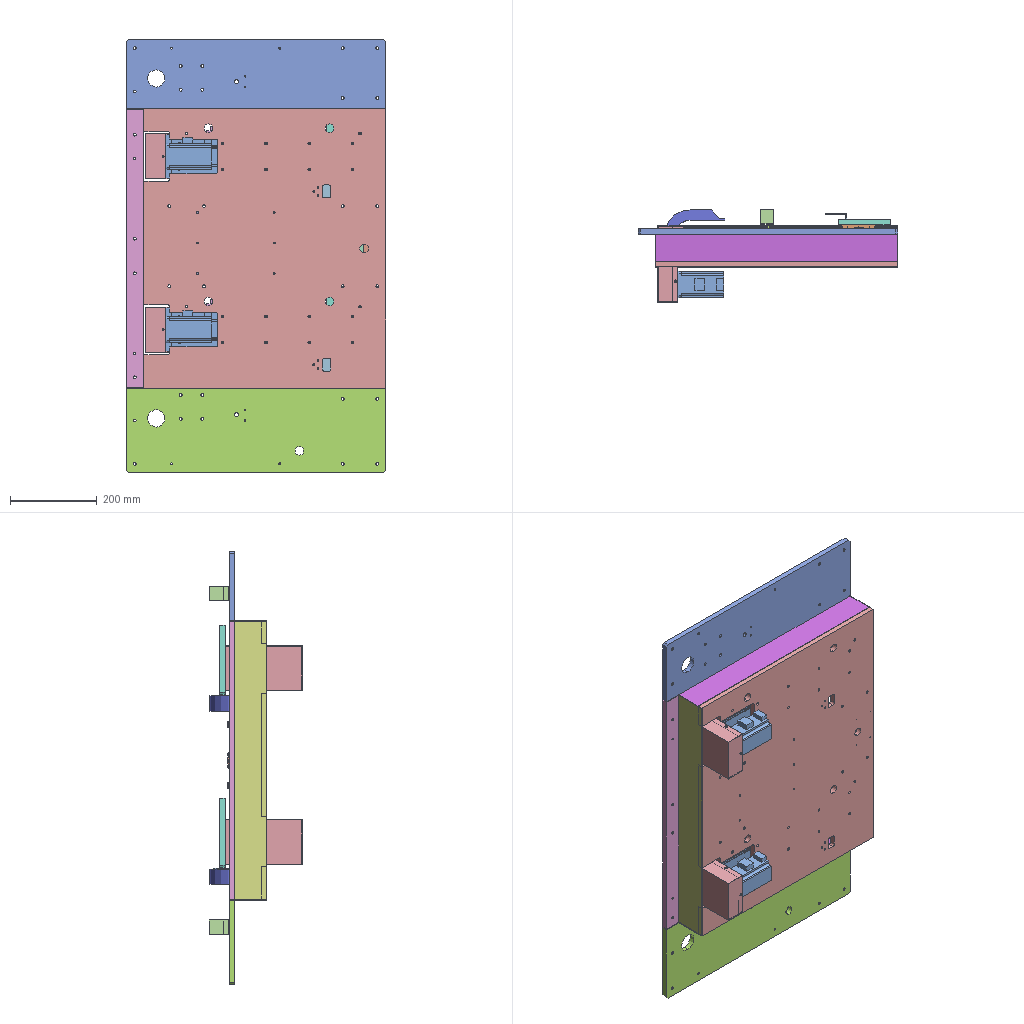Assembly | SolidWorks | 21 different items | 32 placed | box 600 x 215 x 1000 mm
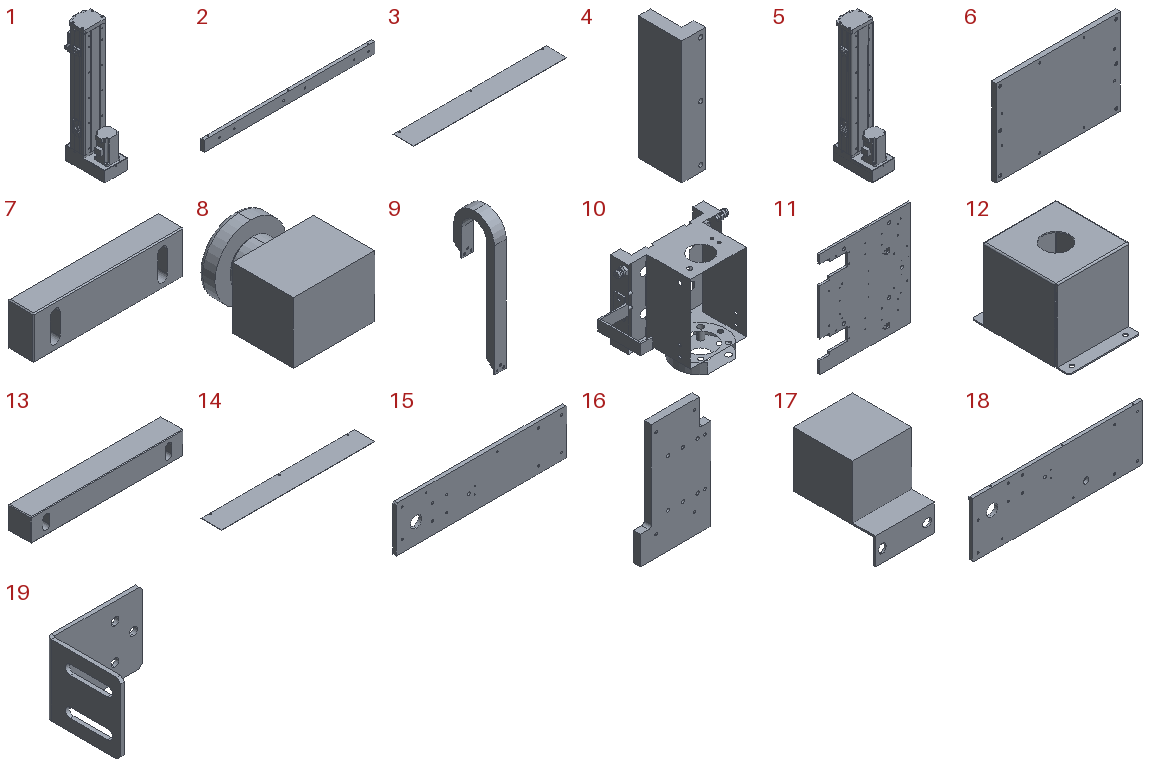Parts list (item | name | quantity | parent item | size | volume | features):
1 | (subassembly) | x2 | - | - | - | -
2 | - | x1 | - | 642 x 12 x 40 mm | 304076 mm3 | features 3DProfileFeature 3, HoleWzd 3, Extrusion 1
3 | - | x1 | - | 642 x 87 x 1 mm | 55806 mm3 | features Cut 1, Extrusion 1
4 | - | x2 | - | 30 x 55 x 156 mm | 162115 mm3 | features 3DProfileFeature 1, Cut 1, Extrusion 1, HoleWzd 1
5 | - | x2 | in 1 | - | - | features RefSurface 11
6 | - | x1 | - | 225 x 8 x 156 mm | 277140 mm3 | features 3DProfileFeature 3, HoleWzd 3, MirrorPattern 3, Extrusion 1
7 | - | x2 | - | 70 x 12 x 20 mm | 15288 mm3 | features Chamfer 1, Cut 1, Extrusion 1
8 | - | x1 | - | 40 x 49 x 35 mm | 47522 mm3 | features Boss 3, Cut 1, Extrusion 1, Fillet 1, LibraryFeature 1
9 | - | x2 | - | 35 x 119.5 x 389.75 mm | 194419 mm3 | features 3DProfileFeature 2, Boss 2, HoleWzd 2, Rib 2, MirrorPattern 1, Sweep 1
10 | - | x2 | in 1 | - | - | features RefSurface 11
11 | - | x1 | - | 559 x 12 x 645 mm | 3901978 mm3 | features Cut 7, 3DProfileFeature 4, HoleWzd 4, Fillet 2, Extrusion 1, LPattern 1
12 | - | x1 | - | 62 x 82 x 62 mm | 18974 mm3 | features EdgeFlange 3, Cut 2, Fillet 1, FlatPattern 1, MirrorPattern 1, SMBaseFlange 1, SheetMetal 1
13 | - | x2 | - | 100 x 15 x 15 mm | 21284 mm3 | features Chamfer 1, Cut 1, Extrusion 1
14 | - | x2 | - | 560 x 75 x 1 mm | 41952 mm3 | features Cut 1, Extrusion 1
15 | - | x1 | - | 600 x 12 x 160 mm | 1127973 mm3 | features 3DProfileFeature 5, HoleWzd 5, Cut 2, Chamfer 1, Extrusion 1
16 | - | x2 | - | 120 x 12 x 200 mm | 238394 mm3 | features 3DProfileFeature 4, HoleWzd 4, Cut 3, Fillet 2, Boss 1, Extrusion 1
17 | - | x2 | - | 33 x 45.5 x 45 mm | 34601 mm3 | features RefAxis 2, Boss 1, Cut 1, Extrusion 1
18 | - | x1 | - | 600 x 12 x 195 mm | 1376203 mm3 | features 3DProfileFeature 5, HoleWzd 5, Cut 3, Chamfer 1, Extrusion 1
19 | - | x2 | - | 50 x 40 x 38 mm | 6031 mm3 | features Chamfer 1, Cut 1, FlatPattern 1, HoleWzd 1, SMBaseFlange 1, SheetMetal 1
20 | Feeder1 | x1 | - | - | - | -
21 | Turntable | x1 | - | - | - | -
Mates (type | each side: item.copy, entity, surface, feature):
In the top assembly
Coincident | 7.1 face plane Extrude1 | 6.1 face plane Extrude1
Coincident | 7.2 face plane Extrude1 | 6.1 face plane Extrude1
Coincident | 13.1 face plane Extrude1 | 13.2 face plane Extrude1
Coincident | 11.1 face plane Extrude1 | 15.1 face plane Extrude1 | 2 times
Coincident | 15.1 face plane Extrude1 | 18.1 face plane Extrude1
Coincident | 11.1 face plane Extrude1 | 18.1 face plane Extrude1 | 2 times
Coincident | 15.1 face plane Extrude1 | 14.1 face plane Extrude1 | 3 times
Coincident | 18.1 face plane Extrude1 | 14.2 face plane Extrude1 | 3 times
Coincident | 11.1 face plane Extrude1 | 12.1 face plane Edge Flange2
Coincident | 11.1 face plane Extrude1 | 12.1 face plane Edge Flange3
Coincident | 11.1 plane | 12.1 plane
Concentric | 12.1 face cylinder Cut-Extrude1 | 8.1 face cylinder Extrude2
Coincident | 12.1 face plane Base Flange1 | 8.1 face plane Cut-Extrude1
Coincident | 18.1 face plane Extrude1 | 2.1 face plane Extrude1 | 2 times
Coincident | 11.1 plane | 2.1 plane
Coincident | 2.1 face plane Extrude1 | 3.1 face plane Extrude1 | 2 times
Coincident | 2.1 plane | 3.1 plane
Coincident | 13.1 face plane Extrude1 | 6.1 face plane Extrude1
Coincident | 7.2 face plane Extrude1 | 7.1 face plane Extrude1
Coincident | 13.2 face plane Extrude1 | 13.1 face plane Extrude1
Width | 5.1 face plane Surface-Import22 | 5.1 face plane Surface-Import22 | 11.1 face plane Cut-Extrude1 | 11.1 face plane Cut-Extrude1
Coincident | 11.1 face plane Extrude1 | 5.1 face plane Surface-Import23
DistanceDim | 11.1 face plane Extrude1 | 5.1 face plane Surface-Import23
Coincident | 10.1 face plane Surface-Import24 | 16.1 face plane Extrude1
DistanceDim | 10.1 face plane Surface-Import24 | 16.1 face plane Extrude1
Width | 16.1 face plane Extrude1 | 16.1 face plane Extrude1 | 10.1 face plane Surface-Import24 | 10.1 face plane Surface-Import24
Coincident | 16.1 face plane Cut-Extrude2 | 19.1 face plane Base Flange1
DistanceDim | 16.1 face plane Extrude1 | 19.1 face plane Base Flange1
Coincident | 16.1 face plane Extrude1 | 19.1 face plane Base Flange1
DistanceDim | 11.1 face plane Extrude1 | 9.1 face plane Fitting114.4.12PZ-2
Width | 19.1 face plane Base Flange1 | 19.1 face plane Base Flange1 | 9.1 face plane Chain | 9.1 face plane Chain
Coincident | 11.1 face plane Extrude1 | 9.1 face plane Chain
Width | 5.2 face plane Surface-Import22 | 5.2 face plane Surface-Import22 | 11.1 face plane Cut-Extrude1 | 11.1 face plane Cut-Extrude1
Coincident | 11.1 face plane Extrude1 | 5.2 face plane Surface-Import23
Coincident | 5.1 face plane Surface-Import23 | 5.2 face plane Surface-Import23
Coincident | 10.2 face plane Surface-Import24 | 16.2 face plane Extrude1
Width | 16.2 face plane Extrude1 | 16.2 face plane Extrude1 | 10.2 face plane Surface-Import24 | 10.2 face plane Surface-Import24
DistanceDim | 10.2 face plane Surface-Import24 | 16.2 face plane Extrude1
Coincident | 16.2 face plane Cut-Extrude2 | 19.2 face plane Base Flange1
DistanceDim | 16.2 face plane Extrude1 | 19.2 face plane Base Flange1
Coincident | 16.2 face plane Extrude1 | 19.2 face plane Base Flange1
Coincident | 11.1 face plane Extrude1 | 9.2 face plane Chain
Coincident | 9.1 face plane Fitting114.4.12PZ-2 | 9.2 face plane Fitting114.4.12PZ-2
Width | 19.2 face plane Base Flange1 | 19.2 face plane Base Flange1 | 9.2 face plane Chain | 9.2 face plane Chain
DistanceDim | 11.1 face plane Extrude1 | 15.1 face plane Extrude1
Coincident | 11.1 face plane Extrude1 | 4.1 face plane Extrude1
Coincident | 4.1 face plane Extrude1 | 6.1 face plane Extrude1 | 2 times
Width | 6.1 face plane Extrude1 | 6.1 face plane Extrude1 | 4.1 face plane Extrude1 | 4.1 face plane Extrude1
Coincident | 4.1 face plane Extrude1 | 4.2 face plane Extrude1
Coincident | 11.1 face plane Extrude1 | 4.2 face plane Extrude1
Coincident | 6.1 face plane Extrude1 | 4.2 face plane Extrude1
Coincident | 15.1 face plane Extrude1 | 17.1 face plane Extrude2
Concentric | 15.1 face cylinder M4 Tapped Hole2 | 17.1 axis | 2 times
Concentric | 18.1 face cylinder M4 Tapped Hole2 | 17.2 axis | 2 times
Coincident | 18.1 face plane Extrude1 | 17.2 face plane Extrude2
In subassembly 1
Width | 5.3 face plane Surface-Import23 | 5.3 face plane Surface-Import23 | 10.3 face plane Surface-Import24 | 10.3 face plane Surface-Import24
DistanceDim | 5.3 face plane Surface-Import23 | 10.3 face plane Surface-Import24
LimitDistanceDim | 5.3 face plane Surface-Import22 | 10.3 face plane Surface-Import24